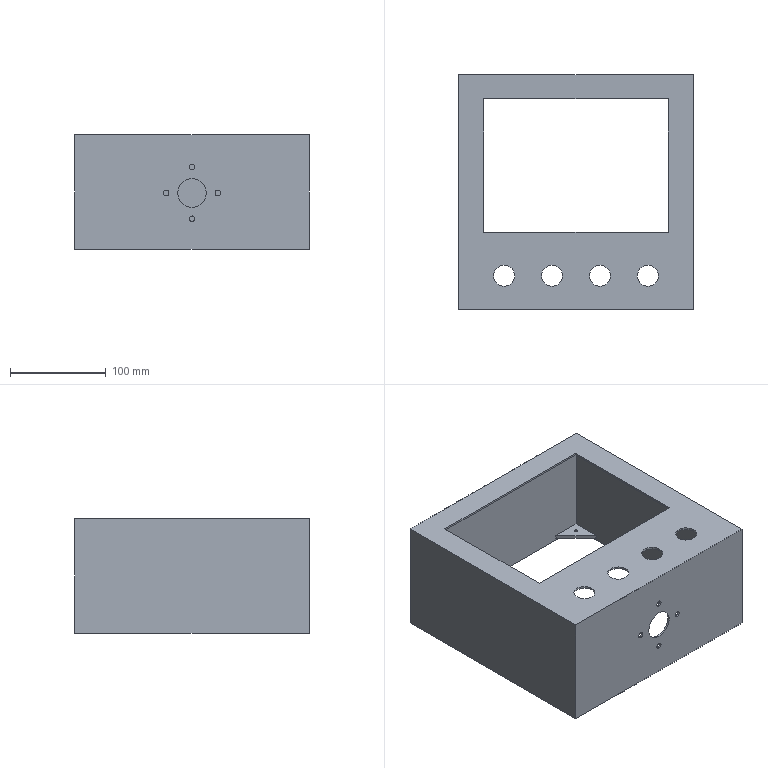Part | STEP file | Sheet metal box | 1 solid | 61 faces | box 245 x 245 x 120 mm | volume 296398 mm3 | plane 27 | cylinder 26 | cone 8 | commonest cylinder face diameters 3.3 x8 6 x8 22 x8 30 x2